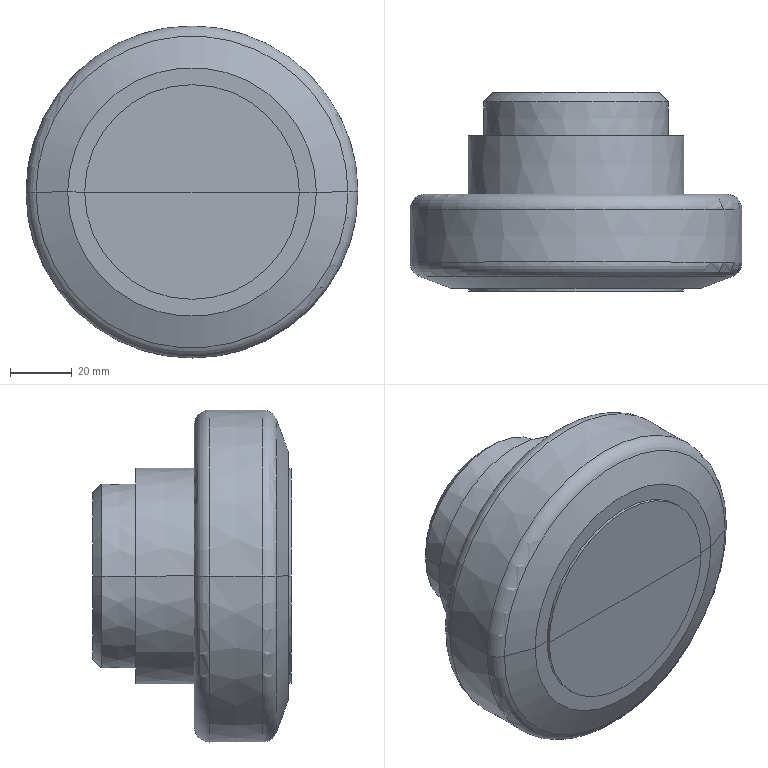Part | SolidWorks | features Revolution 1 | 1 solid | 26 faces | box 107.698 x 64.478 x 107.698 mm | volume 380558 mm3 | cone 22 | torus 4